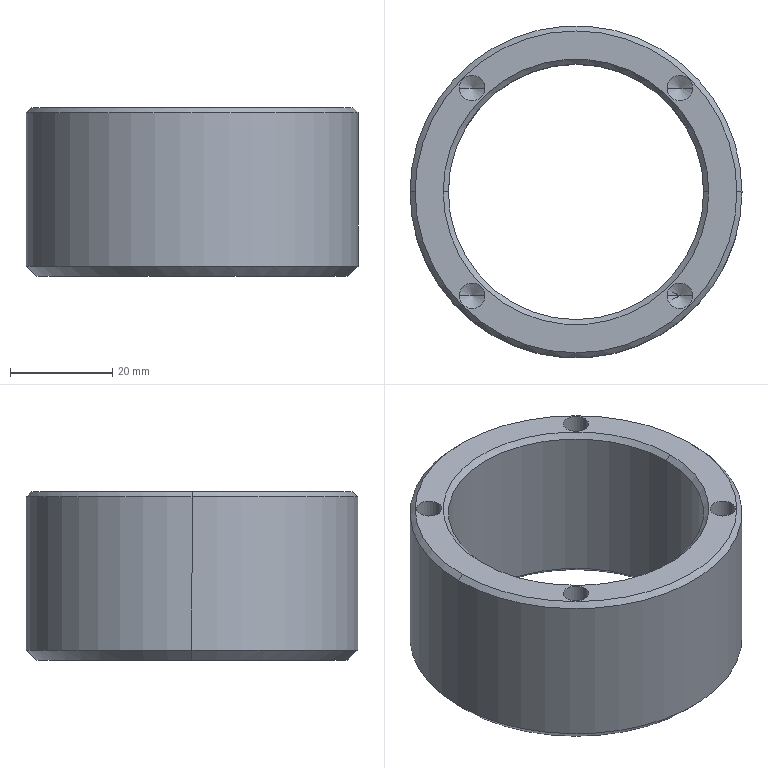Part | STEP file | Locating post-10P30 | 1 solid | 30 faces | box 65 x 65 x 33 mm | volume 42831 mm3 | cone 16 | cylinder 12 | plane 2 | commonest cylinder face diameters 5 x8 50 x2 65 x2